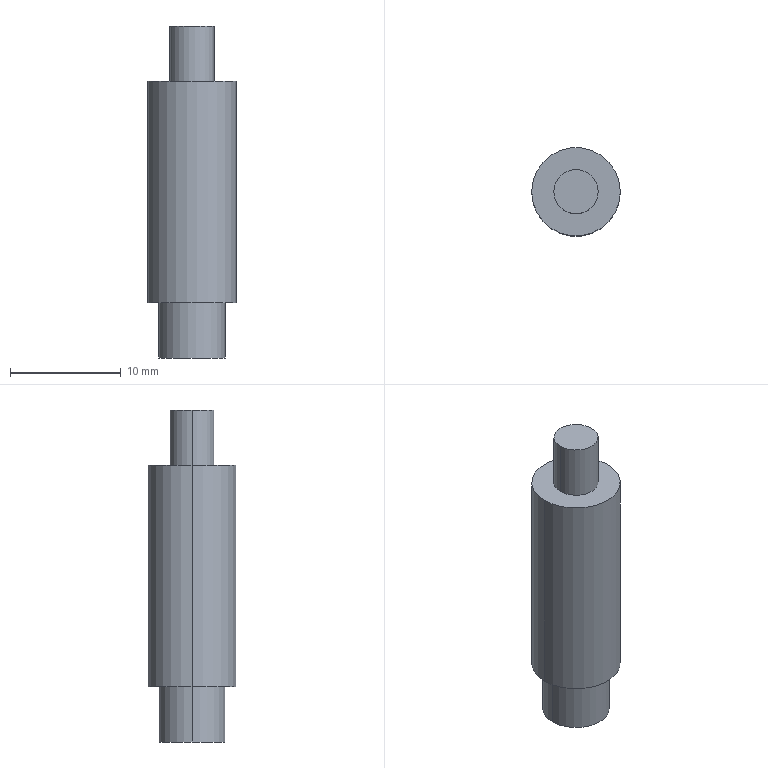Part | STEP file | Proximity m8 | 1 solid | 10 faces | box 8 x 8 x 30 mm | volume 1210 mm3 | cylinder 6 | plane 4 | commonest cylinder face diameters 4 x2 6 x2 8 x2
STEP:
#1=CARTESIAN_POINT('',(0.,0.,0.));
#2=DIRECTION('',(0.,0.,1.));
#3=DIRECTION('',(1.,0.,0.));
#4=AXIS2_PLACEMENT_3D('',#1,#2,#3);
#5=CARTESIAN_POINT('',(-4.,0.,25.));
#6=VERTEX_POINT('',#5);
#7=CARTESIAN_POINT('',(4.,0.,25.));
#8=VERTEX_POINT('',#7);
#9=CARTESIAN_POINT('',(0.,0.,25.));
#10=DIRECTION('',(0.,0.,-1.));
#11=DIRECTION('',(-1.,0.,0.));
#12=AXIS2_PLACEMENT_3D('',#9,#10,#11);
#13=CIRCLE('',#12,4.);
#14=CARTESIAN_POINT('',(0.,0.,25.));
#15=DIRECTION('',(0.,0.,-1.));
#16=DIRECTION('',(-1.,0.,0.));
#17=AXIS2_PLACEMENT_3D('',#14,#15,#16);
#18=CYLINDRICAL_SURFACE('',#17,4.);
#19=CARTESIAN_POINT('',(0.,0.));
#20=DIRECTION('',(1.,0.));
#21=VECTOR('',#20,1.);
#22=LINE('',#19,#21);
#23=(GEOMETRIC_REPRESENTATION_CONTEXT(2)PARAMETRIC_REPRESENTATION_CONTEXT()REPRESENTATION_CONTEXT('',''));
#24=DEFINITIONAL_REPRESENTATION('',(#22),#23);
#25=PCURVE('',#18,#24);
#26=CARTESIAN_POINT('',(0.,0.,25.));
#27=DIRECTION('',(0.,0.,1.));
#28=DIRECTION('',(1.,0.,0.));
#29=AXIS2_PLACEMENT_3D('',#26,#27,#28);
#30=PLANE('',#29);
#31=CARTESIAN_POINT('',(-4.,0.));
#32=CARTESIAN_POINT('',(-4.,6.928));
#33=CARTESIAN_POINT('',(2.,3.464));
#34=CARTESIAN_POINT('',(8.,0.));
#35=CARTESIAN_POINT('',(2.,-3.464));
#36=CARTESIAN_POINT('',(-4.,-6.928));
#37=CARTESIAN_POINT('',(-4.,0.));
#38=(BOUNDED_CURVE()B_SPLINE_CURVE(2,(#31,#32,#33,#34,#35,#36,#37),.UNSPECIFIED.,.T.,.F.)B_SPLINE_CURVE_WITH_KNOTS((1,2,2,2,2,1),(-2.094,0.,2.094,4.189,6.283,8.378),.UNSPECIFIED.)CURVE()GEOMETRIC_REPRESENTATION_ITEM()RATIONAL_B_SPLINE_CURVE((1.,0.5,1.,0.5,1.,0.5,1.))REPRESENTATION_ITEM(''));
#39=(GEOMETRIC_REPRESENTATION_CONTEXT(2)PARAMETRIC_REPRESENTATION_CONTEXT()REPRESENTATION_CONTEXT('',''));
#40=DEFINITIONAL_REPRESENTATION('',(#38),#39);
#41=PCURVE('',#30,#40);
#42=SURFACE_CURVE('',#13,(#25,#41),.PCURVE_S1.);
#43=EDGE_CURVE('',#6,#8,#42,.T.);
#44=ORIENTED_EDGE('',*,*,#43,.T.);
#45=CARTESIAN_POINT('',(4.,0.,5.));
#46=VERTEX_POINT('',#45);
#47=CARTESIAN_POINT('',(4.,0.,25.));
#48=DIRECTION('',(0.,0.,-1.));
#49=VECTOR('',#48,1.);
#50=LINE('',#47,#49);
#51=CARTESIAN_POINT('',(3.142,0.));
#52=DIRECTION('',(0.,1.));
#53=VECTOR('',#52,1.);
#54=LINE('',#51,#53);
#55=(GEOMETRIC_REPRESENTATION_CONTEXT(2)PARAMETRIC_REPRESENTATION_CONTEXT()REPRESENTATION_CONTEXT('',''));
#56=DEFINITIONAL_REPRESENTATION('',(#54),#55);
#57=PCURVE('',#18,#56);
#58=CARTESIAN_POINT('',(0.,0.,25.));
#59=DIRECTION('',(0.,0.,-1.));
#60=DIRECTION('',(-1.,0.,0.));
#61=AXIS2_PLACEMENT_3D('',#58,#59,#60);
#62=CYLINDRICAL_SURFACE('',#61,4.);
#63=CARTESIAN_POINT('',(3.142,0.));
#64=DIRECTION('',(0.,1.));
#65=VECTOR('',#64,1.);
#66=LINE('',#63,#65);
#67=(GEOMETRIC_REPRESENTATION_CONTEXT(2)PARAMETRIC_REPRESENTATION_CONTEXT()REPRESENTATION_CONTEXT('',''));
#68=DEFINITIONAL_REPRESENTATION('',(#66),#67);
#69=PCURVE('',#62,#68);
#70=SURFACE_CURVE('',#50,(#57,#69),.PCURVE_S1.);
#71=EDGE_CURVE('',#8,#46,#70,.T.);
#72=ORIENTED_EDGE('',*,*,#71,.T.);
#73=CARTESIAN_POINT('',(-4.,0.,5.));
#74=VERTEX_POINT('',#73);
#75=CARTESIAN_POINT('',(0.,0.,5.));
#76=DIRECTION('',(0.,0.,1.));
#77=DIRECTION('',(-1.,0.,0.));
#78=AXIS2_PLACEMENT_3D('',#75,#76,#77);
#79=CIRCLE('',#78,4.);
#80=CARTESIAN_POINT('',(6.283,20.));
#81=DIRECTION('',(-1.,0.));
#82=VECTOR('',#81,1.);
#83=LINE('',#80,#82);
#84=(GEOMETRIC_REPRESENTATION_CONTEXT(2)PARAMETRIC_REPRESENTATION_CONTEXT()REPRESENTATION_CONTEXT('',''));
#85=DEFINITIONAL_REPRESENTATION('',(#83),#84);
#86=PCURVE('',#18,#85);
#87=CARTESIAN_POINT('',(0.,0.,5.));
#88=DIRECTION('',(0.,0.,1.));
#89=DIRECTION('',(1.,0.,0.));
#90=AXIS2_PLACEMENT_3D('',#87,#88,#89);
#91=PLANE('',#90);
#92=CARTESIAN_POINT('',(0.,0.));
#93=DIRECTION('',(-1.,0.));
#94=AXIS2_PLACEMENT_2D('',#92,#93);
#95=CIRCLE('',#94,4.);
#96=(GEOMETRIC_REPRESENTATION_CONTEXT(2)PARAMETRIC_REPRESENTATION_CONTEXT()REPRESENTATION_CONTEXT('',''));
#97=DEFINITIONAL_REPRESENTATION('',(#95),#96);
#98=PCURVE('',#91,#97);
#99=SURFACE_CURVE('',#79,(#86,#98),.PCURVE_S1.);
#100=EDGE_CURVE('',#46,#74,#99,.T.);
#101=ORIENTED_EDGE('',*,*,#100,.T.);
#102=CARTESIAN_POINT('',(-4.,0.,25.));
#103=DIRECTION('',(0.,0.,-1.));
#104=VECTOR('',#103,1.);
#105=LINE('',#102,#104);
#106=CARTESIAN_POINT('',(0.,0.));
#107=DIRECTION('',(0.,1.));
#108=VECTOR('',#107,1.);
#109=LINE('',#106,#108);
#110=(GEOMETRIC_REPRESENTATION_CONTEXT(2)PARAMETRIC_REPRESENTATION_CONTEXT()REPRESENTATION_CONTEXT('',''));
#111=DEFINITIONAL_REPRESENTATION('',(#109),#110);
#112=PCURVE('',#18,#111);
#113=CARTESIAN_POINT('',(6.283,0.));
#114=DIRECTION('',(0.,1.));
#115=VECTOR('',#114,1.);
#116=LINE('',#113,#115);
#117=(GEOMETRIC_REPRESENTATION_CONTEXT(2)PARAMETRIC_REPRESENTATION_CONTEXT()REPRESENTATION_CONTEXT('',''));
#118=DEFINITIONAL_REPRESENTATION('',(#116),#117);
#119=PCURVE('',#62,#118);
#120=SURFACE_CURVE('',#105,(#112,#119),.PCURVE_S1.);
#121=EDGE_CURVE('',#6,#74,#120,.T.);
#122=ORIENTED_EDGE('',*,*,#121,.F.);
#123=EDGE_LOOP('',(#44,#72,#101,#122));
#124=FACE_BOUND('',#123,.T.);
#125=ADVANCED_FACE('',(#124),#18,.T.);
#126=CARTESIAN_POINT('',(-3.,0.,5.));
#127=VERTEX_POINT('',#126);
#128=CARTESIAN_POINT('',(3.,0.,5.));
#129=VERTEX_POINT('',#128);
#130=CARTESIAN_POINT('',(0.,0.,5.));
#131=DIRECTION('',(0.,0.,-1.));
#132=DIRECTION('',(-1.,0.,0.));
#133=AXIS2_PLACEMENT_3D('',#130,#131,#132);
#134=CIRCLE('',#133,3.);
#135=CARTESIAN_POINT('',(0.,0.,5.));
#136=DIRECTION('',(0.,0.,-1.));
#137=DIRECTION('',(-1.,0.,0.));
#138=AXIS2_PLACEMENT_3D('',#135,#136,#137);
#139=CYLINDRICAL_SURFACE('',#138,3.);
#140=CARTESIAN_POINT('',(0.,0.));
#141=DIRECTION('',(1.,0.));
#142=VECTOR('',#141,1.);
#143=LINE('',#140,#142);
#144=(GEOMETRIC_REPRESENTATION_CONTEXT(2)PARAMETRIC_REPRESENTATION_CONTEXT()REPRESENTATION_CONTEXT('',''));
#145=DEFINITIONAL_REPRESENTATION('',(#143),#144);
#146=PCURVE('',#139,#145);
#147=CARTESIAN_POINT('',(-3.,0.));
#148=CARTESIAN_POINT('',(-3.,5.196));
#149=CARTESIAN_POINT('',(1.5,2.598));
#150=CARTESIAN_POINT('',(6.,0.));
#151=CARTESIAN_POINT('',(1.5,-2.598));
#152=CARTESIAN_POINT('',(-3.,-5.196));
#153=CARTESIAN_POINT('',(-3.,0.));
#154=(BOUNDED_CURVE()B_SPLINE_CURVE(2,(#147,#148,#149,#150,#151,#152,#153),.UNSPECIFIED.,.T.,.F.)B_SPLINE_CURVE_WITH_KNOTS((1,2,2,2,2,1),(-2.094,0.,2.094,4.189,6.283,8.378),.UNSPECIFIED.)CURVE()GEOMETRIC_REPRESENTATION_ITEM()RATIONAL_B_SPLINE_CURVE((1.,0.5,1.,0.5,1.,0.5,1.))REPRESENTATION_ITEM(''));
#155=(GEOMETRIC_REPRESENTATION_CONTEXT(2)PARAMETRIC_REPRESENTATION_CONTEXT()REPRESENTATION_CONTEXT('',''));
#156=DEFINITIONAL_REPRESENTATION('',(#154),#155);
#157=PCURVE('',#91,#156);
#158=SURFACE_CURVE('',#134,(#146,#157),.PCURVE_S1.);
#159=EDGE_CURVE('',#127,#129,#158,.T.);
#160=ORIENTED_EDGE('',*,*,#159,.T.);
#161=CARTESIAN_POINT('',(3.,0.,0.));
#162=VERTEX_POINT('',#161);
#163=CARTESIAN_POINT('',(3.,0.,5.));
#164=DIRECTION('',(0.,0.,-1.));
#165=VECTOR('',#164,1.);
#166=LINE('',#163,#165);
#167=CARTESIAN_POINT('',(3.142,0.));
#168=DIRECTION('',(0.,1.));
#169=VECTOR('',#168,1.);
#170=LINE('',#167,#169);
#171=(GEOMETRIC_REPRESENTATION_CONTEXT(2)PARAMETRIC_REPRESENTATION_CONTEXT()REPRESENTATION_CONTEXT('',''));
#172=DEFINITIONAL_REPRESENTATION('',(#170),#171);
#173=PCURVE('',#139,#172);
#174=CARTESIAN_POINT('',(0.,0.,5.));
#175=DIRECTION('',(0.,0.,-1.));
#176=DIRECTION('',(-1.,0.,0.));
#177=AXIS2_PLACEMENT_3D('',#174,#175,#176);
#178=CYLINDRICAL_SURFACE('',#177,3.);
#179=CARTESIAN_POINT('',(3.142,0.));
#180=DIRECTION('',(0.,1.));
#181=VECTOR('',#180,1.);
#182=LINE('',#179,#181);
#183=(GEOMETRIC_REPRESENTATION_CONTEXT(2)PARAMETRIC_REPRESENTATION_CONTEXT()REPRESENTATION_CONTEXT('',''));
#184=DEFINITIONAL_REPRESENTATION('',(#182),#183);
#185=PCURVE('',#178,#184);
#186=SURFACE_CURVE('',#166,(#173,#185),.PCURVE_S1.);
#187=EDGE_CURVE('',#129,#162,#186,.T.);
#188=ORIENTED_EDGE('',*,*,#187,.T.);
#189=CARTESIAN_POINT('',(-3.,0.,0.));
#190=VERTEX_POINT('',#189);
#191=CARTESIAN_POINT('',(0.,0.,0.));
#192=DIRECTION('',(0.,0.,1.));
#193=DIRECTION('',(-1.,0.,0.));
#194=AXIS2_PLACEMENT_3D('',#191,#192,#193);
#195=CIRCLE('',#194,3.);
#196=CARTESIAN_POINT('',(6.283,5.));
#197=DIRECTION('',(-1.,0.));
#198=VECTOR('',#197,1.);
#199=LINE('',#196,#198);
#200=(GEOMETRIC_REPRESENTATION_CONTEXT(2)PARAMETRIC_REPRESENTATION_CONTEXT()REPRESENTATION_CONTEXT('',''));
#201=DEFINITIONAL_REPRESENTATION('',(#199),#200);
#202=PCURVE('',#139,#201);
#203=CARTESIAN_POINT('',(0.,0.,0.));
#204=DIRECTION('',(0.,0.,1.));
#205=DIRECTION('',(1.,0.,0.));
#206=AXIS2_PLACEMENT_3D('',#203,#204,#205);
#207=PLANE('',#206);
#208=CARTESIAN_POINT('',(0.,0.));
#209=DIRECTION('',(-1.,0.));
#210=AXIS2_PLACEMENT_2D('',#208,#209);
#211=CIRCLE('',#210,3.);
#212=(GEOMETRIC_REPRESENTATION_CONTEXT(2)PARAMETRIC_REPRESENTATION_CONTEXT()REPRESENTATION_CONTEXT('',''));
#213=DEFINITIONAL_REPRESENTATION('',(#211),#212);
#214=PCURVE('',#207,#213);
#215=SURFACE_CURVE('',#195,(#202,#214),.PCURVE_S1.);
#216=EDGE_CURVE('',#162,#190,#215,.T.);
#217=ORIENTED_EDGE('',*,*,#216,.T.);
#218=CARTESIAN_POINT('',(-3.,0.,5.));
#219=DIRECTION('',(0.,0.,-1.));
#220=VECTOR('',#219,1.);
#221=LINE('',#218,#220);
#222=CARTESIAN_POINT('',(0.,0.));
#223=DIRECTION('',(0.,1.));
#224=VECTOR('',#223,1.);
#225=LINE('',#222,#224);
#226=(GEOMETRIC_REPRESENTATION_CONTEXT(2)PARAMETRIC_REPRESENTATION_CONTEXT()REPRESENTATION_CONTEXT('',''));
#227=DEFINITIONAL_REPRESENTATION('',(#225),#226);
#228=PCURVE('',#139,#227);
#229=CARTESIAN_POINT('',(6.283,0.));
#230=DIRECTION('',(0.,1.));
#231=VECTOR('',#230,1.);
#232=LINE('',#229,#231);
#233=(GEOMETRIC_REPRESENTATION_CONTEXT(2)PARAMETRIC_REPRESENTATION_CONTEXT()REPRESENTATION_CONTEXT('',''));
#234=DEFINITIONAL_REPRESENTATION('',(#232),#233);
#235=PCURVE('',#178,#234);
#236=SURFACE_CURVE('',#221,(#228,#235),.PCURVE_S1.);
#237=EDGE_CURVE('',#127,#190,#236,.T.);
#238=ORIENTED_EDGE('',*,*,#237,.F.);
#239=EDGE_LOOP('',(#160,#188,#217,#238));
#240=FACE_BOUND('',#239,.T.);
#241=ADVANCED_FACE('',(#240),#139,.T.);
#242=CARTESIAN_POINT('',(-2.,0.,30.));
#243=VERTEX_POINT('',#242);
#244=CARTESIAN_POINT('',(2.,0.,30.));
#245=VERTEX_POINT('',#244);
#246=CARTESIAN_POINT('',(0.,0.,30.));
#247=DIRECTION('',(0.,0.,-1.));
#248=DIRECTION('',(-1.,0.,0.));
#249=AXIS2_PLACEMENT_3D('',#246,#247,#248);
#250=CIRCLE('',#249,2.);
#251=CARTESIAN_POINT('',(0.,0.,30.));
#252=DIRECTION('',(0.,0.,-1.));
#253=DIRECTION('',(-1.,0.,0.));
#254=AXIS2_PLACEMENT_3D('',#251,#252,#253);
#255=CYLINDRICAL_SURFACE('',#254,2.);
#256=CARTESIAN_POINT('',(0.,0.));
#257=DIRECTION('',(1.,0.));
#258=VECTOR('',#257,1.);
#259=LINE('',#256,#258);
#260=(GEOMETRIC_REPRESENTATION_CONTEXT(2)PARAMETRIC_REPRESENTATION_CONTEXT()REPRESENTATION_CONTEXT('',''));
#261=DEFINITIONAL_REPRESENTATION('',(#259),#260);
#262=PCURVE('',#255,#261);
#263=CARTESIAN_POINT('',(0.,0.,30.));
#264=DIRECTION('',(0.,0.,1.));
#265=DIRECTION('',(1.,0.,0.));
#266=AXIS2_PLACEMENT_3D('',#263,#264,#265);
#267=PLANE('',#266);
#268=CARTESIAN_POINT('',(-2.,0.));
#269=CARTESIAN_POINT('',(-2.,3.464));
#270=CARTESIAN_POINT('',(1.,1.732));
#271=CARTESIAN_POINT('',(4.,0.));
#272=CARTESIAN_POINT('',(1.,-1.732));
#273=CARTESIAN_POINT('',(-2.,-3.464));
#274=CARTESIAN_POINT('',(-2.,0.));
#275=(BOUNDED_CURVE()B_SPLINE_CURVE(2,(#268,#269,#270,#271,#272,#273,#274),.UNSPECIFIED.,.T.,.F.)B_SPLINE_CURVE_WITH_KNOTS((1,2,2,2,2,1),(-2.094,0.,2.094,4.189,6.283,8.378),.UNSPECIFIED.)CURVE()GEOMETRIC_REPRESENTATION_ITEM()RATIONAL_B_SPLINE_CURVE((1.,0.5,1.,0.5,1.,0.5,1.))REPRESENTATION_ITEM(''));
#276=(GEOMETRIC_REPRESENTATION_CONTEXT(2)PARAMETRIC_REPRESENTATION_CONTEXT()REPRESENTATION_CONTEXT('',''));
#277=DEFINITIONAL_REPRESENTATION('',(#275),#276);
#278=PCURVE('',#267,#277);
#279=SURFACE_CURVE('',#250,(#262,#278),.PCURVE_S1.);
#280=EDGE_CURVE('',#243,#245,#279,.T.);
#281=ORIENTED_EDGE('',*,*,#280,.T.);
#282=CARTESIAN_POINT('',(2.,0.,25.));
#283=VERTEX_POINT('',#282);
#284=CARTESIAN_POINT('',(2.,0.,30.));
#285=DIRECTION('',(0.,0.,-1.));
#286=VECTOR('',#285,1.);
#287=LINE('',#284,#286);
#288=CARTESIAN_POINT('',(3.142,0.));
#289=DIRECTION('',(0.,1.));
#290=VECTOR('',#289,1.);
#291=LINE('',#288,#290);
#292=(GEOMETRIC_REPRESENTATION_CONTEXT(2)PARAMETRIC_REPRESENTATION_CONTEXT()REPRESENTATION_CONTEXT('',''));
#293=DEFINITIONAL_REPRESENTATION('',(#291),#292);
#294=PCURVE('',#255,#293);
#295=CARTESIAN_POINT('',(0.,0.,30.));
#296=DIRECTION('',(0.,0.,-1.));
#297=DIRECTION('',(-1.,0.,0.));
#298=AXIS2_PLACEMENT_3D('',#295,#296,#297);
#299=CYLINDRICAL_SURFACE('',#298,2.);
#300=CARTESIAN_POINT('',(3.142,0.));
#301=DIRECTION('',(0.,1.));
#302=VECTOR('',#301,1.);
#303=LINE('',#300,#302);
#304=(GEOMETRIC_REPRESENTATION_CONTEXT(2)PARAMETRIC_REPRESENTATION_CONTEXT()REPRESENTATION_CONTEXT('',''));
#305=DEFINITIONAL_REPRESENTATION('',(#303),#304);
#306=PCURVE('',#299,#305);
#307=SURFACE_CURVE('',#287,(#294,#306),.PCURVE_S1.);
#308=EDGE_CURVE('',#245,#283,#307,.T.);
#309=ORIENTED_EDGE('',*,*,#308,.T.);
#310=CARTESIAN_POINT('',(-2.,0.,25.));
#311=VERTEX_POINT('',#310);
#312=CARTESIAN_POINT('',(0.,0.,25.));
#313=DIRECTION('',(0.,0.,-1.));
#314=DIRECTION('',(-1.,0.,0.));
#315=AXIS2_PLACEMENT_3D('',#312,#313,#314);
#316=CIRCLE('',#315,2.);
#317=CARTESIAN_POINT('',(0.,5.));
#318=DIRECTION('',(1.,0.));
#319=VECTOR('',#318,1.);
#320=LINE('',#317,#319);
#321=(GEOMETRIC_REPRESENTATION_CONTEXT(2)PARAMETRIC_REPRESENTATION_CONTEXT()REPRESENTATION_CONTEXT('',''));
#322=DEFINITIONAL_REPRESENTATION('',(#320),#321);
#323=PCURVE('',#255,#322);
#324=CARTESIAN_POINT('',(-2.,0.));
#325=CARTESIAN_POINT('',(-2.,3.464));
#326=CARTESIAN_POINT('',(1.,1.732));
#327=CARTESIAN_POINT('',(4.,0.));
#328=CARTESIAN_POINT('',(1.,-1.732));
#329=CARTESIAN_POINT('',(-2.,-3.464));
#330=CARTESIAN_POINT('',(-2.,0.));
#331=(BOUNDED_CURVE()B_SPLINE_CURVE(2,(#324,#325,#326,#327,#328,#329,#330),.UNSPECIFIED.,.T.,.F.)B_SPLINE_CURVE_WITH_KNOTS((1,2,2,2,2,1),(-2.094,0.,2.094,4.189,6.283,8.378),.UNSPECIFIED.)CURVE()GEOMETRIC_REPRESENTATION_ITEM()RATIONAL_B_SPLINE_CURVE((1.,0.5,1.,0.5,1.,0.5,1.))REPRESENTATION_ITEM(''));
#332=(GEOMETRIC_REPRESENTATION_CONTEXT(2)PARAMETRIC_REPRESENTATION_CONTEXT()REPRESENTATION_CONTEXT('',''));
#333=DEFINITIONAL_REPRESENTATION('',(#331),#332);
#334=PCURVE('',#30,#333);
#335=SURFACE_CURVE('',#316,(#323,#334),.PCURVE_S1.);
#336=EDGE_CURVE('',#311,#283,#335,.T.);
#337=ORIENTED_EDGE('',*,*,#336,.F.);
#338=CARTESIAN_POINT('',(-2.,0.,30.));
#339=DIRECTION('',(0.,0.,-1.));
#340=VECTOR('',#339,1.);
#341=LINE('',#338,#340);
#342=CARTESIAN_POINT('',(0.,0.));
#343=DIRECTION('',(0.,1.));
#344=VECTOR('',#343,1.);
#345=LINE('',#342,#344);
#346=(GEOMETRIC_REPRESENTATION_CONTEXT(2)PARAMETRIC_REPRESENTATION_CONTEXT()REPRESENTATION_CONTEXT('',''));
#347=DEFINITIONAL_REPRESENTATION('',(#345),#346);
#348=PCURVE('',#255,#347);
#349=CARTESIAN_POINT('',(6.283,0.));
#350=DIRECTION('',(0.,1.));
#351=VECTOR('',#350,1.);
#352=LINE('',#349,#351);
#353=(GEOMETRIC_REPRESENTATION_CONTEXT(2)PARAMETRIC_REPRESENTATION_CONTEXT()REPRESENTATION_CONTEXT('',''));
#354=DEFINITIONAL_REPRESENTATION('',(#352),#353);
#355=PCURVE('',#299,#354);
#356=SURFACE_CURVE('',#341,(#348,#355),.PCURVE_S1.);
#357=EDGE_CURVE('',#243,#311,#356,.T.);
#358=ORIENTED_EDGE('',*,*,#357,.F.);
#359=EDGE_LOOP('',(#281,#309,#337,#358));
#360=FACE_BOUND('',#359,.T.);
#361=ADVANCED_FACE('',(#360),#255,.T.);
#362=ORIENTED_EDGE('',*,*,#71,.F.);
#363=CARTESIAN_POINT('',(0.,0.,25.));
#364=DIRECTION('',(0.,0.,-1.));
#365=DIRECTION('',(-1.,0.,0.));
#366=AXIS2_PLACEMENT_3D('',#363,#364,#365);
#367=CIRCLE('',#366,4.);
#368=CARTESIAN_POINT('',(0.,0.));
#369=DIRECTION('',(1.,0.));
#370=VECTOR('',#369,1.);
#371=LINE('',#368,#370);
#372=(GEOMETRIC_REPRESENTATION_CONTEXT(2)PARAMETRIC_REPRESENTATION_CONTEXT()REPRESENTATION_CONTEXT('',''));
#373=DEFINITIONAL_REPRESENTATION('',(#371),#372);
#374=PCURVE('',#62,#373);
#375=CARTESIAN_POINT('',(-4.,0.));
#376=CARTESIAN_POINT('',(-4.,6.928));
#377=CARTESIAN_POINT('',(2.,3.464));
#378=CARTESIAN_POINT('',(8.,0.));
#379=CARTESIAN_POINT('',(2.,-3.464));
#380=CARTESIAN_POINT('',(-4.,-6.928));
#381=CARTESIAN_POINT('',(-4.,0.));
#382=(BOUNDED_CURVE()B_SPLINE_CURVE(2,(#375,#376,#377,#378,#379,#380,#381),.UNSPECIFIED.,.T.,.F.)B_SPLINE_CURVE_WITH_KNOTS((1,2,2,2,2,1),(-2.094,0.,2.094,4.189,6.283,8.378),.UNSPECIFIED.)CURVE()GEOMETRIC_REPRESENTATION_ITEM()RATIONAL_B_SPLINE_CURVE((1.,0.5,1.,0.5,1.,0.5,1.))REPRESENTATION_ITEM(''));
#383=(GEOMETRIC_REPRESENTATION_CONTEXT(2)PARAMETRIC_REPRESENTATION_CONTEXT()REPRESENTATION_CONTEXT('',''));
#384=DEFINITIONAL_REPRESENTATION('',(#382),#383);
#385=PCURVE('',#30,#384);
#386=SURFACE_CURVE('',#367,(#374,#385),.PCURVE_S1.);
#387=EDGE_CURVE('',#8,#6,#386,.T.);
#388=ORIENTED_EDGE('',*,*,#387,.T.);
#389=ORIENTED_EDGE('',*,*,#121,.T.);
#390=CARTESIAN_POINT('',(0.,0.,5.));
#391=DIRECTION('',(0.,0.,1.));
#392=DIRECTION('',(-1.,0.,0.));
#393=AXIS2_PLACEMENT_3D('',#390,#391,#392);
#394=CIRCLE('',#393,4.);
#395=CARTESIAN_POINT('',(6.283,20.));
#396=DIRECTION('',(-1.,0.));
#397=VECTOR('',#396,1.);
#398=LINE('',#395,#397);
#399=(GEOMETRIC_REPRESENTATION_CONTEXT(2)PARAMETRIC_REPRESENTATION_CONTEXT()REPRESENTATION_CONTEXT('',''));
#400=DEFINITIONAL_REPRESENTATION('',(#398),#399);
#401=PCURVE('',#62,#400);
#402=CARTESIAN_POINT('',(0.,0.));
#403=DIRECTION('',(-1.,0.));
#404=AXIS2_PLACEMENT_2D('',#402,#403);
#405=CIRCLE('',#404,4.);
#406=(GEOMETRIC_REPRESENTATION_CONTEXT(2)PARAMETRIC_REPRESENTATION_CONTEXT()REPRESENTATION_CONTEXT('',''));
#407=DEFINITIONAL_REPRESENTATION('',(#405),#406);
#408=PCURVE('',#91,#407);
#409=SURFACE_CURVE('',#394,(#401,#408),.PCURVE_S1.);
#410=EDGE_CURVE('',#74,#46,#409,.T.);
#411=ORIENTED_EDGE('',*,*,#410,.T.);
#412=EDGE_LOOP('',(#362,#388,#389,#411));
#413=FACE_BOUND('',#412,.T.);
#414=ADVANCED_FACE('',(#413),#62,.T.);
#415=ORIENTED_EDGE('',*,*,#159,.F.);
#416=CARTESIAN_POINT('',(0.,0.,5.));
#417=DIRECTION('',(0.,0.,-1.));
#418=DIRECTION('',(-1.,0.,0.));
#419=AXIS2_PLACEMENT_3D('',#416,#417,#418);
#420=CIRCLE('',#419,3.);
#421=CARTESIAN_POINT('',(-3.,0.));
#422=CARTESIAN_POINT('',(-3.,5.196));
#423=CARTESIAN_POINT('',(1.5,2.598));
#424=CARTESIAN_POINT('',(6.,0.));
#425=CARTESIAN_POINT('',(1.5,-2.598));
#426=CARTESIAN_POINT('',(-3.,-5.196));
#427=CARTESIAN_POINT('',(-3.,0.));
#428=(BOUNDED_CURVE()B_SPLINE_CURVE(2,(#421,#422,#423,#424,#425,#426,#427),.UNSPECIFIED.,.T.,.F.)B_SPLINE_CURVE_WITH_KNOTS((1,2,2,2,2,1),(-2.094,0.,2.094,4.189,6.283,8.378),.UNSPECIFIED.)CURVE()GEOMETRIC_REPRESENTATION_ITEM()RATIONAL_B_SPLINE_CURVE((1.,0.5,1.,0.5,1.,0.5,1.))REPRESENTATION_ITEM(''));
#429=(GEOMETRIC_REPRESENTATION_CONTEXT(2)PARAMETRIC_REPRESENTATION_CONTEXT()REPRESENTATION_CONTEXT('',''));
#430=DEFINITIONAL_REPRESENTATION('',(#428),#429);
#431=PCURVE('',#91,#430);
#432=CARTESIAN_POINT('',(0.,0.));
#433=DIRECTION('',(1.,0.));
#434=VECTOR('',#433,1.);
#435=LINE('',#432,#434);
#436=(GEOMETRIC_REPRESENTATION_CONTEXT(2)PARAMETRIC_REPRESENTATION_CONTEXT()REPRESENTATION_CONTEXT('',''));
#437=DEFINITIONAL_REPRESENTATION('',(#435),#436);
#438=PCURVE('',#178,#437);
#439=SURFACE_CURVE('',#420,(#431,#438),.PCURVE_S1.);
#440=EDGE_CURVE('',#129,#127,#439,.T.);
#441=ORIENTED_EDGE('',*,*,#440,.F.);
#442=EDGE_LOOP('',(#415,#441));
#443=FACE_BOUND('',#442,.T.);
#444=ORIENTED_EDGE('',*,*,#410,.F.);
#445=ORIENTED_EDGE('',*,*,#100,.F.);
#446=EDGE_LOOP('',(#444,#445));
#447=FACE_BOUND('',#446,.T.);
#448=ADVANCED_FACE('',(#443,#447),#91,.F.);
#449=ORIENTED_EDGE('',*,*,#336,.T.);
#450=CARTESIAN_POINT('',(0.,0.,25.));
#451=DIRECTION('',(0.,0.,-1.));
#452=DIRECTION('',(-1.,0.,0.));
#453=AXIS2_PLACEMENT_3D('',#450,#451,#452);
#454=CIRCLE('',#453,2.);
#455=CARTESIAN_POINT('',(-2.,0.));
#456=CARTESIAN_POINT('',(-2.,3.464));
#457=CARTESIAN_POINT('',(1.,1.732));
#458=CARTESIAN_POINT('',(4.,0.));
#459=CARTESIAN_POINT('',(1.,-1.732));
#460=CARTESIAN_POINT('',(-2.,-3.464));
#461=CARTESIAN_POINT('',(-2.,0.));
#462=(BOUNDED_CURVE()B_SPLINE_CURVE(2,(#455,#456,#457,#458,#459,#460,#461),.UNSPECIFIED.,.T.,.F.)B_SPLINE_CURVE_WITH_KNOTS((1,2,2,2,2,1),(-2.094,0.,2.094,4.189,6.283,8.378),.UNSPECIFIED.)CURVE()GEOMETRIC_REPRESENTATION_ITEM()RATIONAL_B_SPLINE_CURVE((1.,0.5,1.,0.5,1.,0.5,1.))REPRESENTATION_ITEM(''));
#463=(GEOMETRIC_REPRESENTATION_CONTEXT(2)PARAMETRIC_REPRESENTATION_CONTEXT()REPRESENTATION_CONTEXT('',''));
#464=DEFINITIONAL_REPRESENTATION('',(#462),#463);
#465=PCURVE('',#30,#464);
#466=CARTESIAN_POINT('',(0.,5.));
#467=DIRECTION('',(1.,0.));
#468=VECTOR('',#467,1.);
#469=LINE('',#466,#468);
#470=(GEOMETRIC_REPRESENTATION_CONTEXT(2)PARAMETRIC_REPRESENTATION_CONTEXT()REPRESENTATION_CONTEXT('',''));
#471=DEFINITIONAL_REPRESENTATION('',(#469),#470);
#472=PCURVE('',#299,#471);
#473=SURFACE_CURVE('',#454,(#465,#472),.PCURVE_S1.);
#474=EDGE_CURVE('',#283,#311,#473,.T.);
#475=ORIENTED_EDGE('',*,*,#474,.T.);
#476=EDGE_LOOP('',(#449,#475));
#477=FACE_BOUND('',#476,.T.);
#478=ORIENTED_EDGE('',*,*,#43,.F.);
#479=ORIENTED_EDGE('',*,*,#387,.F.);
#480=EDGE_LOOP('',(#478,#479));
#481=FACE_BOUND('',#480,.T.);
#482=ADVANCED_FACE('',(#477,#481),#30,.T.);
#483=ORIENTED_EDGE('',*,*,#187,.F.);
#484=ORIENTED_EDGE('',*,*,#440,.T.);
#485=ORIENTED_EDGE('',*,*,#237,.T.);
#486=CARTESIAN_POINT('',(0.,0.,0.));
#487=DIRECTION('',(0.,0.,1.));
#488=DIRECTION('',(-1.,0.,0.));
#489=AXIS2_PLACEMENT_3D('',#486,#487,#488);
#490=CIRCLE('',#489,3.);
#491=CARTESIAN_POINT('',(6.283,5.));
#492=DIRECTION('',(-1.,0.));
#493=VECTOR('',#492,1.);
#494=LINE('',#491,#493);
#495=(GEOMETRIC_REPRESENTATION_CONTEXT(2)PARAMETRIC_REPRESENTATION_CONTEXT()REPRESENTATION_CONTEXT('',''));
#496=DEFINITIONAL_REPRESENTATION('',(#494),#495);
#497=PCURVE('',#178,#496);
#498=CARTESIAN_POINT('',(0.,0.));
#499=DIRECTION('',(-1.,0.));
#500=AXIS2_PLACEMENT_2D('',#498,#499);
#501=CIRCLE('',#500,3.);
#502=(GEOMETRIC_REPRESENTATION_CONTEXT(2)PARAMETRIC_REPRESENTATION_CONTEXT()REPRESENTATION_CONTEXT('',''));
#503=DEFINITIONAL_REPRESENTATION('',(#501),#502);
#504=PCURVE('',#207,#503);
#505=SURFACE_CURVE('',#490,(#497,#504),.PCURVE_S1.);
#506=EDGE_CURVE('',#190,#162,#505,.T.);
#507=ORIENTED_EDGE('',*,*,#506,.T.);
#508=EDGE_LOOP('',(#483,#484,#485,#507));
#509=FACE_BOUND('',#508,.T.);
#510=ADVANCED_FACE('',(#509),#178,.T.);
#511=ORIENTED_EDGE('',*,*,#308,.F.);
#512=CARTESIAN_POINT('',(0.,0.,30.));
#513=DIRECTION('',(0.,0.,-1.));
#514=DIRECTION('',(-1.,0.,0.));
#515=AXIS2_PLACEMENT_3D('',#512,#513,#514);
#516=CIRCLE('',#515,2.);
#517=CARTESIAN_POINT('',(0.,0.));
#518=DIRECTION('',(1.,0.));
#519=VECTOR('',#518,1.);
#520=LINE('',#517,#519);
#521=(GEOMETRIC_REPRESENTATION_CONTEXT(2)PARAMETRIC_REPRESENTATION_CONTEXT()REPRESENTATION_CONTEXT('',''));
#522=DEFINITIONAL_REPRESENTATION('',(#520),#521);
#523=PCURVE('',#299,#522);
#524=CARTESIAN_POINT('',(-2.,0.));
#525=CARTESIAN_POINT('',(-2.,3.464));
#526=CARTESIAN_POINT('',(1.,1.732));
#527=CARTESIAN_POINT('',(4.,0.));
#528=CARTESIAN_POINT('',(1.,-1.732));
#529=CARTESIAN_POINT('',(-2.,-3.464));
#530=CARTESIAN_POINT('',(-2.,0.));
#531=(BOUNDED_CURVE()B_SPLINE_CURVE(2,(#524,#525,#526,#527,#528,#529,#530),.UNSPECIFIED.,.T.,.F.)B_SPLINE_CURVE_WITH_KNOTS((1,2,2,2,2,1),(-2.094,0.,2.094,4.189,6.283,8.378),.UNSPECIFIED.)CURVE()GEOMETRIC_REPRESENTATION_ITEM()RATIONAL_B_SPLINE_CURVE((1.,0.5,1.,0.5,1.,0.5,1.))REPRESENTATION_ITEM(''));
#532=(GEOMETRIC_REPRESENTATION_CONTEXT(2)PARAMETRIC_REPRESENTATION_CONTEXT()REPRESENTATION_CONTEXT('',''));
#533=DEFINITIONAL_REPRESENTATION('',(#531),#532);
#534=PCURVE('',#267,#533);
#535=SURFACE_CURVE('',#516,(#523,#534),.PCURVE_S1.);
#536=EDGE_CURVE('',#245,#243,#535,.T.);
#537=ORIENTED_EDGE('',*,*,#536,.T.);
#538=ORIENTED_EDGE('',*,*,#357,.T.);
#539=ORIENTED_EDGE('',*,*,#474,.F.);
#540=EDGE_LOOP('',(#511,#537,#538,#539));
#541=FACE_BOUND('',#540,.T.);
#542=ADVANCED_FACE('',(#541),#299,.T.);
#543=ORIENTED_EDGE('',*,*,#506,.F.);
#544=ORIENTED_EDGE('',*,*,#216,.F.);
#545=EDGE_LOOP('',(#543,#544));
#546=FACE_BOUND('',#545,.T.);
#547=ADVANCED_FACE('',(#546),#207,.F.);
#548=ORIENTED_EDGE('',*,*,#280,.F.);
#549=ORIENTED_EDGE('',*,*,#536,.F.);
#550=EDGE_LOOP('',(#548,#549));
#551=FACE_BOUND('',#550,.T.);
#552=ADVANCED_FACE('',(#551),#267,.T.);
#553=CLOSED_SHELL('',(#125,#241,#361,#414,#448,#482,#510,#542,#547,#552));
#554=MANIFOLD_SOLID_BREP('',#553);
#555=(LENGTH_UNIT()NAMED_UNIT(*)SI_UNIT(.MILLI.,.METRE.));
#556=UNCERTAINTY_MEASURE_WITH_UNIT(LENGTH_MEASURE(0.0000001),#555,'','');
#557=(NAMED_UNIT(*)PLANE_ANGLE_UNIT()SI_UNIT($,.RADIAN.));
#558=(NAMED_UNIT(*)SI_UNIT($,.STERADIAN.)SOLID_ANGLE_UNIT());
#559=(GEOMETRIC_REPRESENTATION_CONTEXT(3)GLOBAL_UNCERTAINTY_ASSIGNED_CONTEXT((#556))GLOBAL_UNIT_ASSIGNED_CONTEXT((#555,#557,#558))REPRESENTATION_CONTEXT('',''));
#560=ADVANCED_BREP_SHAPE_REPRESENTATION('',(#4,#554),#559);